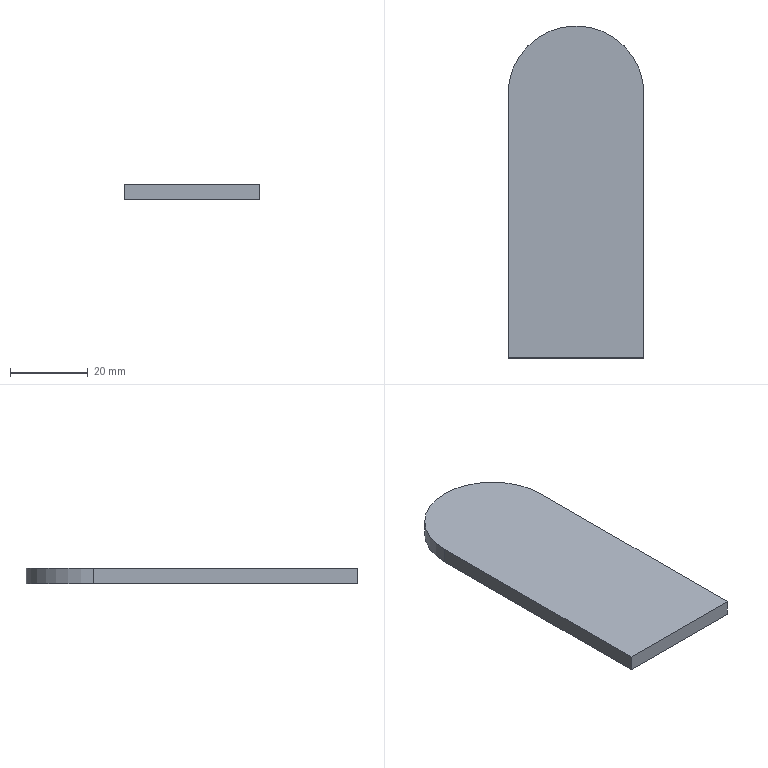Part | SolidWorks | features Extrusion 1 | 1 solid | 6 faces | box 35 x 85.5 x 4 mm | volume 11444 mm3 | plane 5 | cylinder 1 | commonest cylinder face diameters 35 x1
STEP:
#1=CARTESIAN_POINT('',(17.5,0.,0.));
#2=VERTEX_POINT('',#1);
#3=CARTESIAN_POINT('',(17.5,68.,0.));
#4=VERTEX_POINT('',#3);
#5=CARTESIAN_POINT('',(17.5,68.,0.));
#6=DIRECTION('',(0.,1.,0.));
#7=VECTOR('',#6,1000.);
#8=LINE('',#5,#7);
#9=EDGE_CURVE('',#2,#4,#8,.T.);
#10=ORIENTED_EDGE('',*,*,#9,.T.);
#11=CARTESIAN_POINT('',(17.5,68.,4.));
#12=VERTEX_POINT('',#11);
#13=CARTESIAN_POINT('',(17.5,68.,4.));
#14=DIRECTION('',(0.,0.,-1.));
#15=VECTOR('',#14,1000.);
#16=LINE('',#13,#15);
#17=EDGE_CURVE('',#12,#4,#16,.T.);
#18=ORIENTED_EDGE('',*,*,#17,.F.);
#19=CARTESIAN_POINT('',(17.5,0.,4.));
#20=VERTEX_POINT('',#19);
#21=CARTESIAN_POINT('',(17.5,68.,4.));
#22=DIRECTION('',(0.,1.,0.));
#23=VECTOR('',#22,1000.);
#24=LINE('',#21,#23);
#25=EDGE_CURVE('',#20,#12,#24,.T.);
#26=ORIENTED_EDGE('',*,*,#25,.F.);
#27=CARTESIAN_POINT('',(17.5,0.,4.));
#28=DIRECTION('',(0.,0.,-1.));
#29=VECTOR('',#28,1000.);
#30=LINE('',#27,#29);
#31=EDGE_CURVE('',#20,#2,#30,.T.);
#32=ORIENTED_EDGE('',*,*,#31,.T.);
#33=EDGE_LOOP('',(#10,#18,#26,#32));
#34=FACE_OUTER_BOUND('',#33,.T.);
#35=CARTESIAN_POINT('',(17.5,68.,4.));
#36=DIRECTION('',(-1.,0.,0.));
#37=DIRECTION('',(0.,-1.,0.));
#38=AXIS2_PLACEMENT_3D('',#35,#36,#37);
#39=PLANE('',#38);
#40=ADVANCED_FACE('',(#34),#39,.F.);
#41=CARTESIAN_POINT('',(-17.5,68.,0.));
#42=VERTEX_POINT('',#41);
#43=CARTESIAN_POINT('',(0.,68.,0.));
#44=DIRECTION('',(0.,0.,1.));
#45=DIRECTION('',(-1.,0.,0.));
#46=AXIS2_PLACEMENT_3D('',#43,#44,#45);
#47=CIRCLE('',#46,17.5);
#48=EDGE_CURVE('',#4,#42,#47,.T.);
#49=ORIENTED_EDGE('',*,*,#48,.T.);
#50=CARTESIAN_POINT('',(-17.5,68.,4.));
#51=VERTEX_POINT('',#50);
#52=CARTESIAN_POINT('',(-17.5,68.,4.));
#53=DIRECTION('',(0.,0.,-1.));
#54=VECTOR('',#53,1000.);
#55=LINE('',#52,#54);
#56=EDGE_CURVE('',#51,#42,#55,.T.);
#57=ORIENTED_EDGE('',*,*,#56,.F.);
#58=CARTESIAN_POINT('',(0.,68.,4.));
#59=DIRECTION('',(0.,0.,1.));
#60=DIRECTION('',(-1.,0.,0.));
#61=AXIS2_PLACEMENT_3D('',#58,#59,#60);
#62=CIRCLE('',#61,17.5);
#63=EDGE_CURVE('',#12,#51,#62,.T.);
#64=ORIENTED_EDGE('',*,*,#63,.F.);
#65=ORIENTED_EDGE('',*,*,#17,.T.);
#66=EDGE_LOOP('',(#49,#57,#64,#65));
#67=FACE_OUTER_BOUND('',#66,.T.);
#68=CARTESIAN_POINT('',(0.,68.,4.));
#69=DIRECTION('',(0.,0.,-1.));
#70=DIRECTION('',(-1.,0.,0.));
#71=AXIS2_PLACEMENT_3D('',#68,#69,#70);
#72=CYLINDRICAL_SURFACE('',#71,17.5);
#73=ADVANCED_FACE('',(#67),#72,.T.);
#74=CARTESIAN_POINT('',(-17.5,0.,0.));
#75=VERTEX_POINT('',#74);
#76=CARTESIAN_POINT('',(-17.5,0.,0.));
#77=DIRECTION('',(0.,-1.,0.));
#78=VECTOR('',#77,1000.);
#79=LINE('',#76,#78);
#80=EDGE_CURVE('',#42,#75,#79,.T.);
#81=ORIENTED_EDGE('',*,*,#80,.T.);
#82=CARTESIAN_POINT('',(-17.5,0.,4.));
#83=VERTEX_POINT('',#82);
#84=CARTESIAN_POINT('',(-17.5,0.,4.));
#85=DIRECTION('',(0.,0.,-1.));
#86=VECTOR('',#85,1000.);
#87=LINE('',#84,#86);
#88=EDGE_CURVE('',#83,#75,#87,.T.);
#89=ORIENTED_EDGE('',*,*,#88,.F.);
#90=CARTESIAN_POINT('',(-17.5,0.,4.));
#91=DIRECTION('',(0.,-1.,0.));
#92=VECTOR('',#91,1000.);
#93=LINE('',#90,#92);
#94=EDGE_CURVE('',#51,#83,#93,.T.);
#95=ORIENTED_EDGE('',*,*,#94,.F.);
#96=ORIENTED_EDGE('',*,*,#56,.T.);
#97=EDGE_LOOP('',(#81,#89,#95,#96));
#98=FACE_OUTER_BOUND('',#97,.T.);
#99=CARTESIAN_POINT('',(-17.5,0.,4.));
#100=DIRECTION('',(1.,0.,0.));
#101=DIRECTION('',(0.,1.,0.));
#102=AXIS2_PLACEMENT_3D('',#99,#100,#101);
#103=PLANE('',#102);
#104=ADVANCED_FACE('',(#98),#103,.F.);
#105=CARTESIAN_POINT('',(0.,0.,0.));
#106=DIRECTION('',(1.,0.,0.));
#107=VECTOR('',#106,1000.);
#108=LINE('',#105,#107);
#109=EDGE_CURVE('',#75,#2,#108,.T.);
#110=ORIENTED_EDGE('',*,*,#109,.T.);
#111=ORIENTED_EDGE('',*,*,#31,.F.);
#112=CARTESIAN_POINT('',(17.5,0.,4.));
#113=DIRECTION('',(1.,0.,0.));
#114=VECTOR('',#113,1000.);
#115=LINE('',#112,#114);
#116=EDGE_CURVE('',#83,#20,#115,.T.);
#117=ORIENTED_EDGE('',*,*,#116,.F.);
#118=ORIENTED_EDGE('',*,*,#88,.T.);
#119=EDGE_LOOP('',(#110,#111,#117,#118));
#120=FACE_OUTER_BOUND('',#119,.T.);
#121=CARTESIAN_POINT('',(0.,0.,4.));
#122=DIRECTION('',(0.,1.,0.));
#123=DIRECTION('',(-1.,0.,0.));
#124=AXIS2_PLACEMENT_3D('',#121,#122,#123);
#125=PLANE('',#124);
#126=ADVANCED_FACE('',(#120),#125,.F.);
#127=ORIENTED_EDGE('',*,*,#116,.T.);
#128=ORIENTED_EDGE('',*,*,#25,.T.);
#129=ORIENTED_EDGE('',*,*,#63,.T.);
#130=ORIENTED_EDGE('',*,*,#94,.T.);
#131=EDGE_LOOP('',(#127,#128,#129,#130));
#132=FACE_OUTER_BOUND('',#131,.T.);
#133=CARTESIAN_POINT('',(0.,68.,4.));
#134=DIRECTION('',(0.,0.,-1.));
#135=DIRECTION('',(-1.,0.,0.));
#136=AXIS2_PLACEMENT_3D('',#133,#134,#135);
#137=PLANE('',#136);
#138=ADVANCED_FACE('',(#132),#137,.F.);
#139=ORIENTED_EDGE('',*,*,#9,.F.);
#140=ORIENTED_EDGE('',*,*,#109,.F.);
#141=ORIENTED_EDGE('',*,*,#80,.F.);
#142=ORIENTED_EDGE('',*,*,#48,.F.);
#143=EDGE_LOOP('',(#139,#140,#141,#142));
#144=FACE_OUTER_BOUND('',#143,.T.);
#145=CARTESIAN_POINT('',(0.,68.,0.));
#146=DIRECTION('',(0.,0.,-1.));
#147=DIRECTION('',(-1.,0.,0.));
#148=AXIS2_PLACEMENT_3D('',#145,#146,#147);
#149=PLANE('',#148);
#150=ADVANCED_FACE('',(#144),#149,.T.);
#151=CLOSED_SHELL('',(#40,#73,#104,#126,#138,#150));
#152=MANIFOLD_SOLID_BREP('',#151);
#153=CARTESIAN_POINT('',(0.,0.,0.));
#154=DIRECTION('',(0.,0.,1.));
#155=DIRECTION('',(1.,0.,0.));
#156=AXIS2_PLACEMENT_3D('',#153,#154,#155);
#157=(LENGTH_UNIT()NAMED_UNIT(*)SI_UNIT(.MILLI.,.METRE.));
#158=UNCERTAINTY_MEASURE_WITH_UNIT(LENGTH_MEASURE(0.00001),#157,'','');
#159=(NAMED_UNIT(*)PLANE_ANGLE_UNIT()SI_UNIT($,.RADIAN.));
#160=(NAMED_UNIT(*)SI_UNIT($,.STERADIAN.)SOLID_ANGLE_UNIT());
#161=(GEOMETRIC_REPRESENTATION_CONTEXT(3)GLOBAL_UNCERTAINTY_ASSIGNED_CONTEXT((#158))GLOBAL_UNIT_ASSIGNED_CONTEXT((#157,#159,#160))REPRESENTATION_CONTEXT('',''));
#162=ADVANCED_BREP_SHAPE_REPRESENTATION('',(#152,#156),#161);